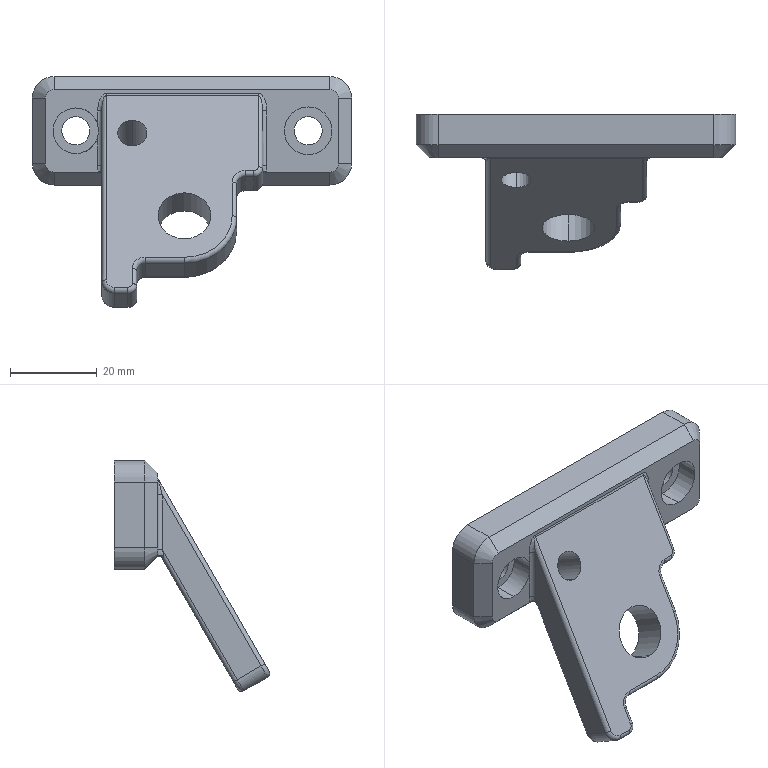Part | SolidWorks | features BaseBody 1 | 1 solid | 85 faces | box 73.5 x 35.728 x 53.18 mm | volume 24950 mm3 | cylinder 40 | plane 21 | torus 12 | spline 8 | cone 4 | commonest cylinder face diameters 2 x18 4 x4 6.5 x4 10 x4 6.8 x2 10.5 x2